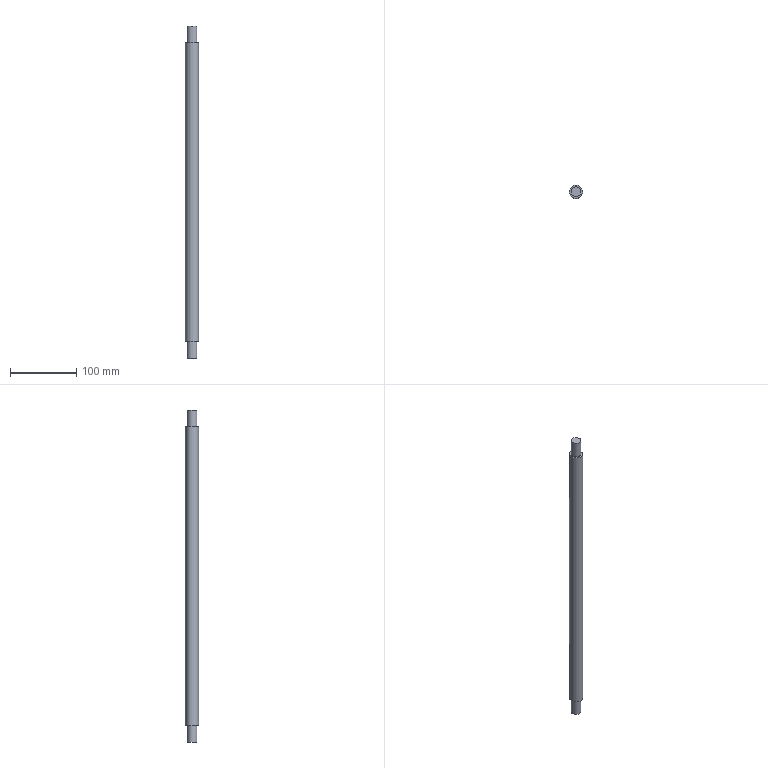Part | NX | features DATUM_CSYS 4, EXTRUDE 3, SKETCH 3 | 1 solid | 7 faces | box 20 x 20 x 500 mm | volume 150207 mm3 | plane 4 | cylinder 3 | commonest cylinder face diameters 15 x2 20 x1
STEP:
#1=CARTESIAN_POINT('',(10.,0.,450.));
#2=VERTEX_POINT('',#1);
#3=CARTESIAN_POINT('',(0.,0.,450.));
#4=DIRECTION('',(0.,0.,1.));
#5=DIRECTION('',(1.,0.,0.));
#6=AXIS2_PLACEMENT_3D('',#3,#4,#5);
#7=CIRCLE('',#6,10.);
#8=EDGE_CURVE('',#2,#2,#7,.T.);
#9=ORIENTED_EDGE('',*,*,#8,.F.);
#10=EDGE_LOOP('',(#9));
#11=FACE_BOUND('',#10,.T.);
#12=CARTESIAN_POINT('',(10.,0.,0.));
#13=VERTEX_POINT('',#12);
#14=CARTESIAN_POINT('',(0.,0.,0.));
#15=DIRECTION('',(0.,0.,1.));
#16=DIRECTION('',(1.,0.,0.));
#17=AXIS2_PLACEMENT_3D('',#14,#15,#16);
#18=CIRCLE('',#17,10.);
#19=EDGE_CURVE('',#13,#13,#18,.T.);
#20=ORIENTED_EDGE('',*,*,#19,.T.);
#21=EDGE_LOOP('',(#20));
#22=FACE_BOUND('',#21,.T.);
#23=CARTESIAN_POINT('',(0.,0.,450.));
#24=DIRECTION('',(0.,0.,-1.));
#25=DIRECTION('',(-1.,0.,0.));
#26=AXIS2_PLACEMENT_3D('',#23,#24,#25);
#27=CYLINDRICAL_SURFACE('',#26,10.);
#28=ADVANCED_FACE('',(#11,#22),#27,.T.);
#29=CARTESIAN_POINT('',(7.5,0.,450.));
#30=VERTEX_POINT('',#29);
#31=CARTESIAN_POINT('',(0.,0.,450.));
#32=DIRECTION('',(0.,0.,1.));
#33=DIRECTION('',(1.,0.,0.));
#34=AXIS2_PLACEMENT_3D('',#31,#32,#33);
#35=CIRCLE('',#34,7.5);
#36=EDGE_CURVE('',#30,#30,#35,.T.);
#37=ORIENTED_EDGE('',*,*,#36,.F.);
#38=EDGE_LOOP('',(#37));
#39=FACE_BOUND('',#38,.T.);
#40=ORIENTED_EDGE('',*,*,#8,.T.);
#41=EDGE_LOOP('',(#40));
#42=FACE_BOUND('',#41,.T.);
#43=CARTESIAN_POINT('',(0.,0.,450.));
#44=DIRECTION('',(0.,0.,1.));
#45=DIRECTION('',(1.,0.,0.));
#46=AXIS2_PLACEMENT_3D('',#43,#44,#45);
#47=PLANE('',#46);
#48=ADVANCED_FACE('',(#39,#42),#47,.T.);
#49=CARTESIAN_POINT('',(7.5,0.,0.));
#50=VERTEX_POINT('',#49);
#51=CARTESIAN_POINT('',(0.,0.,0.));
#52=DIRECTION('',(0.,0.,1.));
#53=DIRECTION('',(1.,0.,0.));
#54=AXIS2_PLACEMENT_3D('',#51,#52,#53);
#55=CIRCLE('',#54,7.5);
#56=EDGE_CURVE('',#50,#50,#55,.F.);
#57=ORIENTED_EDGE('',*,*,#56,.F.);
#58=EDGE_LOOP('',(#57));
#59=FACE_BOUND('',#58,.T.);
#60=ORIENTED_EDGE('',*,*,#19,.F.);
#61=EDGE_LOOP('',(#60));
#62=FACE_BOUND('',#61,.T.);
#63=CARTESIAN_POINT('',(0.,0.,0.));
#64=DIRECTION('',(0.,0.,1.));
#65=DIRECTION('',(1.,0.,0.));
#66=AXIS2_PLACEMENT_3D('',#63,#64,#65);
#67=PLANE('',#66);
#68=ADVANCED_FACE('',(#59,#62),#67,.F.);
#69=CARTESIAN_POINT('',(7.5,0.,-25.));
#70=VERTEX_POINT('',#69);
#71=CARTESIAN_POINT('',(0.,0.,-25.));
#72=DIRECTION('',(0.,0.,-1.));
#73=DIRECTION('',(1.,0.,0.));
#74=AXIS2_PLACEMENT_3D('',#71,#72,#73);
#75=CIRCLE('',#74,7.5);
#76=EDGE_CURVE('',#70,#70,#75,.T.);
#77=ORIENTED_EDGE('',*,*,#76,.F.);
#78=EDGE_LOOP('',(#77));
#79=FACE_BOUND('',#78,.T.);
#80=ORIENTED_EDGE('',*,*,#56,.T.);
#81=EDGE_LOOP('',(#80));
#82=FACE_BOUND('',#81,.T.);
#83=CARTESIAN_POINT('',(0.,0.,-25.));
#84=DIRECTION('',(0.,0.,1.));
#85=DIRECTION('',(1.,0.,0.));
#86=AXIS2_PLACEMENT_3D('',#83,#84,#85);
#87=CYLINDRICAL_SURFACE('',#86,7.5);
#88=ADVANCED_FACE('',(#79,#82),#87,.T.);
#89=ORIENTED_EDGE('',*,*,#76,.T.);
#90=EDGE_LOOP('',(#89));
#91=FACE_BOUND('',#90,.T.);
#92=CARTESIAN_POINT('',(0.,0.,-25.));
#93=DIRECTION('',(0.,0.,-1.));
#94=DIRECTION('',(-1.,0.,0.));
#95=AXIS2_PLACEMENT_3D('',#92,#93,#94);
#96=PLANE('',#95);
#97=ADVANCED_FACE('',(#91),#96,.T.);
#98=ORIENTED_EDGE('',*,*,#36,.T.);
#99=EDGE_LOOP('',(#98));
#100=FACE_BOUND('',#99,.T.);
#101=CARTESIAN_POINT('',(7.5,0.,475.));
#102=VERTEX_POINT('',#101);
#103=CARTESIAN_POINT('',(0.,0.,475.));
#104=DIRECTION('',(0.,0.,1.));
#105=DIRECTION('',(1.,0.,0.));
#106=AXIS2_PLACEMENT_3D('',#103,#104,#105);
#107=CIRCLE('',#106,7.5);
#108=EDGE_CURVE('',#102,#102,#107,.T.);
#109=ORIENTED_EDGE('',*,*,#108,.F.);
#110=EDGE_LOOP('',(#109));
#111=FACE_BOUND('',#110,.T.);
#112=CARTESIAN_POINT('',(0.,0.,475.));
#113=DIRECTION('',(0.,0.,-1.));
#114=DIRECTION('',(-1.,0.,0.));
#115=AXIS2_PLACEMENT_3D('',#112,#113,#114);
#116=CYLINDRICAL_SURFACE('',#115,7.5);
#117=ADVANCED_FACE('',(#100,#111),#116,.T.);
#118=ORIENTED_EDGE('',*,*,#108,.T.);
#119=EDGE_LOOP('',(#118));
#120=FACE_BOUND('',#119,.T.);
#121=CARTESIAN_POINT('',(0.,0.,475.));
#122=DIRECTION('',(0.,0.,1.));
#123=DIRECTION('',(1.,0.,0.));
#124=AXIS2_PLACEMENT_3D('',#121,#122,#123);
#125=PLANE('',#124);
#126=ADVANCED_FACE('',(#120),#125,.T.);
#127=CLOSED_SHELL('',(#28,#48,#68,#88,#97,#117,#126));
#128=MANIFOLD_SOLID_BREP('',#127);
#129=(LENGTH_UNIT()NAMED_UNIT(*)SI_UNIT(.MILLI.,.METRE.));
#130=UNCERTAINTY_MEASURE_WITH_UNIT(LENGTH_MEASURE(0.00001),#129,'','');
#131=(NAMED_UNIT(*)PLANE_ANGLE_UNIT()SI_UNIT($,.RADIAN.));
#132=(NAMED_UNIT(*)SI_UNIT($,.STERADIAN.)SOLID_ANGLE_UNIT());
#133=(GEOMETRIC_REPRESENTATION_CONTEXT(3)GLOBAL_UNCERTAINTY_ASSIGNED_CONTEXT((#130))GLOBAL_UNIT_ASSIGNED_CONTEXT((#129,#131,#132))REPRESENTATION_CONTEXT('',''));
#134=ADVANCED_BREP_SHAPE_REPRESENTATION('',(#128),#133);